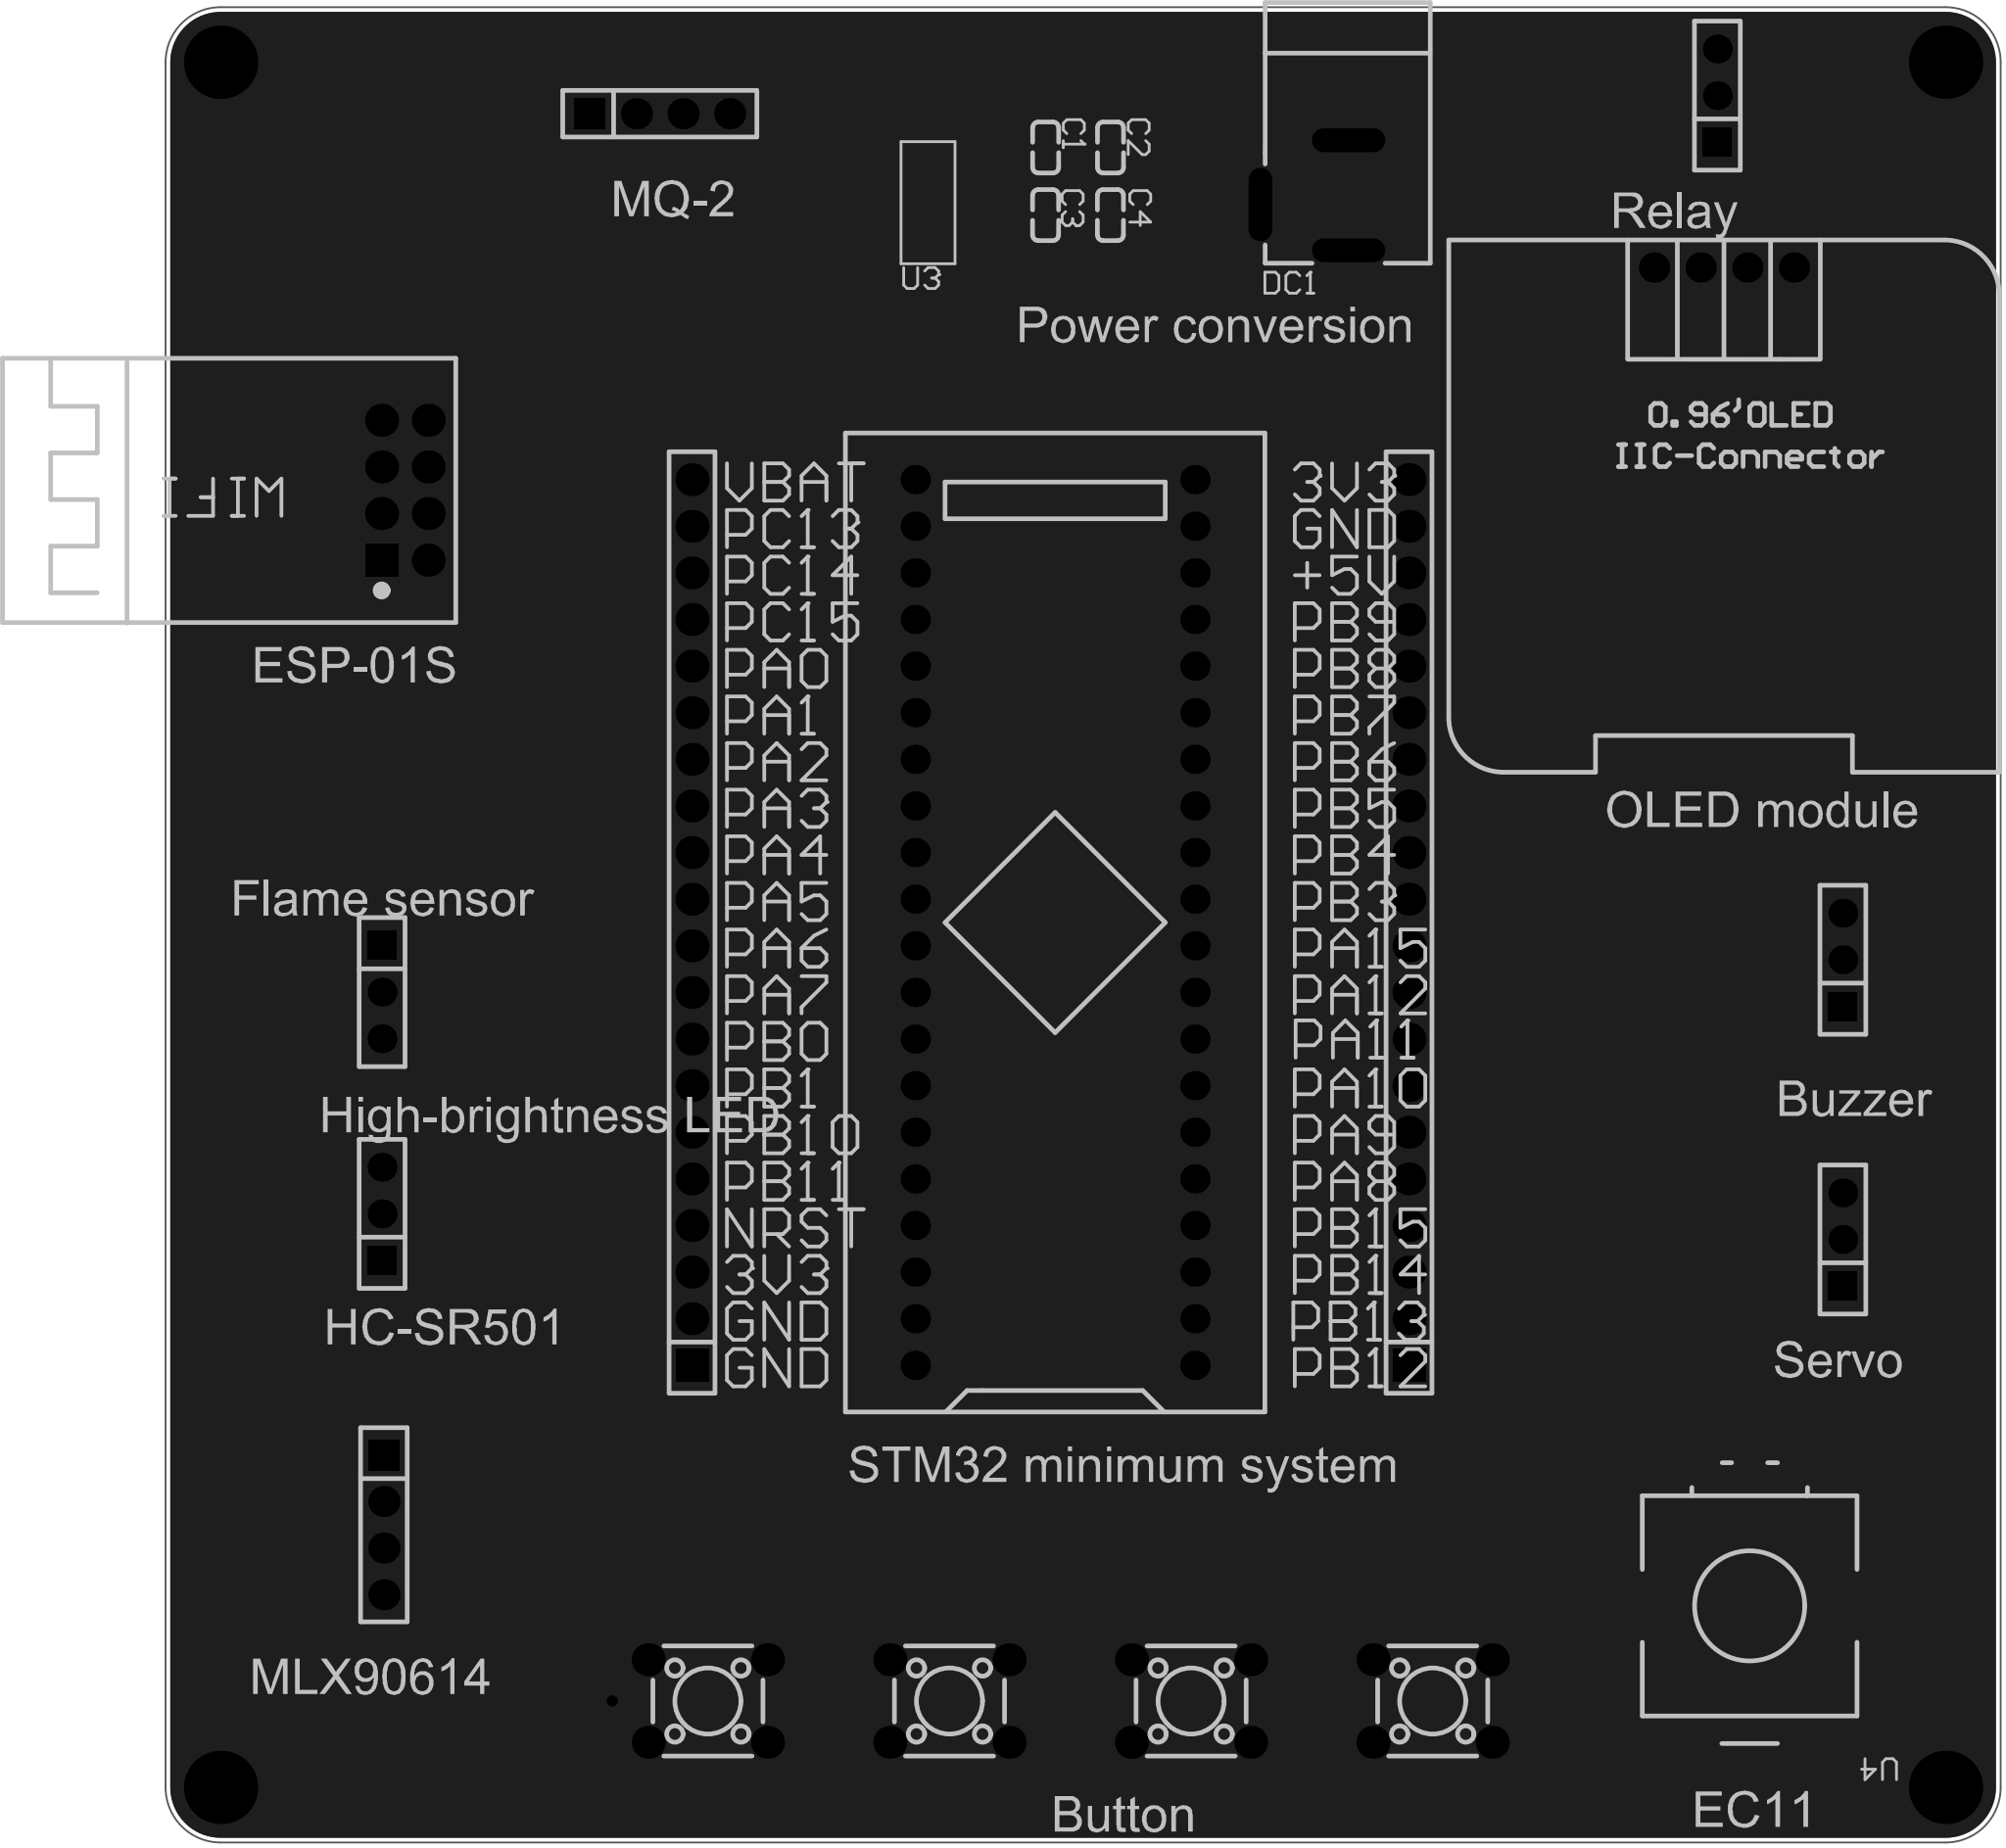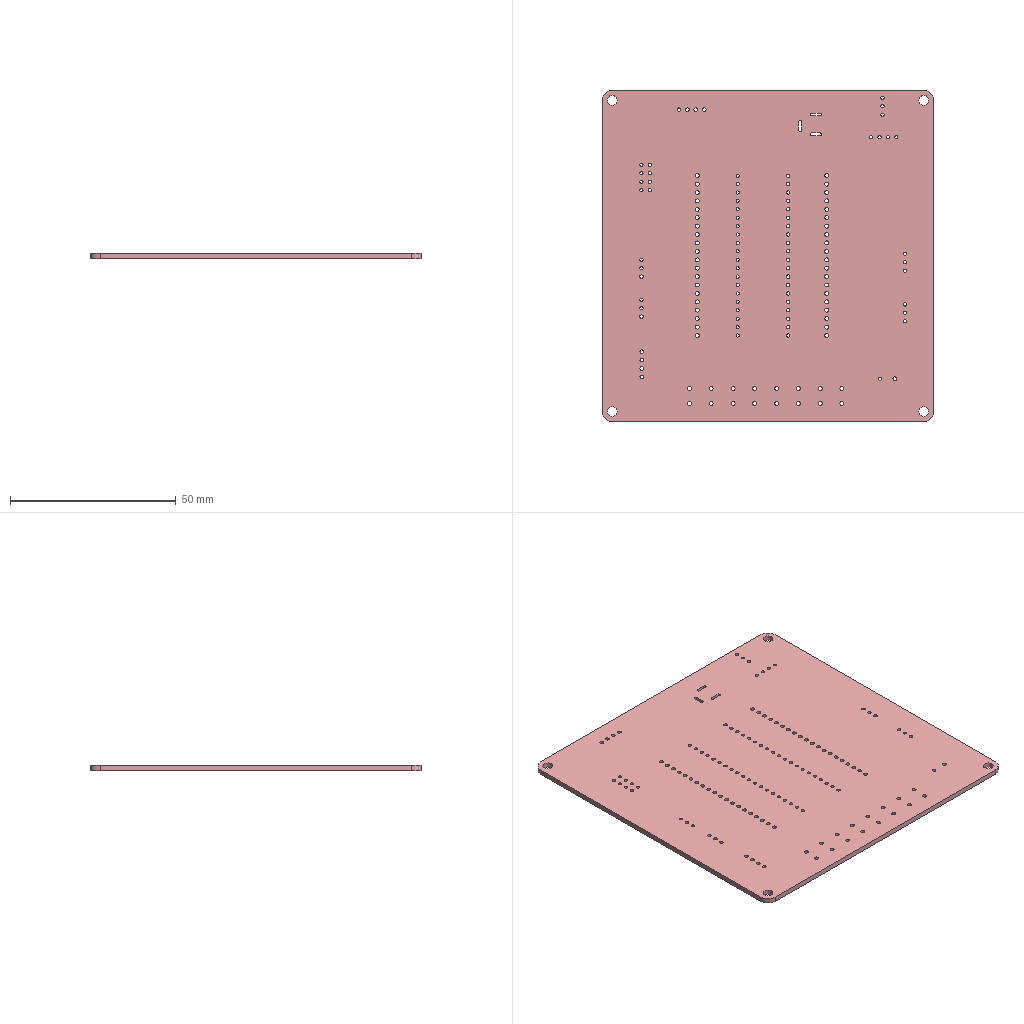Circuit board layout | Altium Designer | box 100 x 100 x 1.6 mm
Layer stack:
# Altium Designer layer stack of  (unit mm; dielectric type: 0 none, 1 core, 2 prepreg, 3 surface material)
index,name,kind,layer,copper_thickness_mm,dielectric_type,dielectric_thickness_mm,dielectric_material,dielectric_constant
0,Top Paste Mask Layer,other,,,,,,
1,Top Silkscreen Layer,other,,,,,,
2,Top Solder Mask Layer,dielectric,,,3,0.01,,3.3
3,Top Layer,copper,Top Layer,0.035,,,,
4,Dielectric1,dielectric,,,3,1.51,FR4,4.5
5,Bottom Layer,copper,Bottom Layer,0.035,,,,
6,Bottom Solder Mask Layer,dielectric,,,3,0.01,,3.3
7,Bottom Silkscreen Layer,other,,,,,,
8,Bottom Paste Mask Layer,other,,,,,,
# drill layer pairs: low layer,high layer
drill_pair,Top Layer,Bottom Layer
Part placement:
Designator,Comment,Layer,Footprint,Center-X(mm),Center-Y(mm),Rotation
U1,STM32F103C8T6-Card,TopLayer,CONN-TH_L53.3-W22.9_STM32F103C8T6-CARD,133.623,129.032,90
H1,,TopLayer,HDR-TH_20P-P2.54-V-F,152.906,129.032,90
H2,,TopLayer,HDR-TH_20P-P2.54-V-F,113.835,129.032,90
OLED1,,TopLayer,0.96OLED_4P,170.072,164.719,0
SW5,,TopLayer,SW-TH_4P-L6.0-W6.0-P4.50-LS6.5,154.197,86.614,0
SW6,,TopLayer,SW-TH_4P-L6.0-W6.0-P4.50-LS6.5,127.866,86.614,0
SW7,,TopLayer,SW-TH_4P-L6.0-W6.0-P4.50-LS6.5,114.7,86.614,0
U2,Ai-Thinker ESP-01S ESP8266,TopLayer,WIFIM-TH_8P-L24.7-W14.4-P2.54,98.19,152.585,180
H10,,TopLayer,HDR-TH_3P-P2.54-V-F,96.945,125.24,270
H11,,TopLayer,HDR-TH_3P-P2.54-V-F,96.945,113.157,90
H12,,TopLayer,HDR-TH_3P-P2.54-V-F,169.71,174.088,90
H13,,TopLayer,HDR-TH_3P-P2.54-V-F,176.549,111.76,90
H6,,TopLayer,HDR-TH_4P-P2.54-V-F,112.078,173.101,0
SW1,,TopLayer,SW-TH_4P-L6.0-W6.0-P4.50-LS6.5,141.031,86.614,0
C1,100nF,TopLayer,C0603,133.105,171.26,270
C2,100nF,TopLayer,C0603,136.639,171.26,270
C3,100nF,TopLayer,C0603,133.101,167.577,90
C4,100nF,TopLayer,C0603,136.635,167.577,90
U3,AMS1117-3.3,TopLayer,SOT-223-3_L6.5-W3.4-P2.30-LS7.0-BR,126.794,168.252,0
DC1,,TopLayer,DC-2.0,147.212,168.656,90
H4,,TopLayer,HDR-TH_3P-P2.54-V-F,176.549,127,90
H5,,TopLayer,HDR-TH_4P-P2.54-V-F,97.044,96.216,270
U4,EC1106S,TopLayer,SW-SMD_EC1106S,171.469,91.948,180
Pad and via stacks:
# Altium Designer via and pad stacks of  (unit mm). Each distinct definition once, with the count of objects using it.
# via: kind,start_layer,end_layer,hole_mm,diameter_mm,mode(0 simple;1 top-mid-bottom;2 full stack),diameter_per_layer,count,example_net
# pad: kind,layer,hole_mm,hole_type(0 round;1 square;2 slot),plating,top_size,top_shape(1 round;2 rect;3 octagon;9 rounded rect),mid_size,bottom_size,mode,footprint,size_per_layer,count,example
pad,Multi-Layer,3,0,plated,4x4,1,4x4,4x4,0,,,4,1
pad,Multi-Layer,1,0,plated,1.6x1.6,1,1.6x1.6,1.6x1.6,0,CONN-TH_L53.3-W22.9_STM32F103C8T6-CARD,,40,U1.1
pad,Multi-Layer,1.2,0,plated,1.8x1.8,2,1.8x1.8,1.8x1.8,0,HDR-TH_20P-P2.54-V-F,,2,H1.1
pad,Multi-Layer,1.2,0,plated,1.8x1.8,1,1.8x1.8,1.8x1.8,0,HDR-TH_20P-P2.54-V-F,,38,H1.2
pad,Multi-Layer,1,0,plated,1.65x1.65,1,1.65x1.65,1.65x1.65,0,0.96OLED_4P,,4,OLED1.4
pad,Multi-Layer,1.2,0,plated,1.8x1.8,1,1.8x1.8,1.8x1.8,0,SW-TH_4P-L6.0-W6.0-P4.50-LS6.5,,16,SW5.1
pad,Multi-Layer,1,0,plated,1.8x1.8,1,1.8x1.8,1.8x1.8,0,WIFIM-TH_8P-L24.7-W14.4-P2.54,,7,U2.8
pad,Multi-Layer,1,0,plated,1.8x1.8,2,1.8x1.8,1.8x1.8,0,WIFIM-TH_8P-L24.7-W14.4-P2.54,,1,U2.1
pad,Multi-Layer,1.02,0,plated,1.575x1.575,1,1.575x1.575,1.575x1.575,0,HDR-TH_3P-P2.54-V-F,,10,H10.3
pad,Multi-Layer,1.02,0,plated,1.575x1.575,2,1.575x1.575,1.575x1.575,0,HDR-TH_3P-P2.54-V-F,,5,H10.1
pad,Multi-Layer,1.1,0,plated,1.7x1.7,2,1.7x1.7,1.7x1.7,0,HDR-TH_4P-P2.54-V-F,,2,H6.1
pad,Multi-Layer,1.1,0,plated,1.7x1.7,1,1.7x1.7,1.7x1.7,0,HDR-TH_4P-P2.54-V-F,,6,H6.2
pad,Multi-Layer,0.8001,2,plated,4x1.3,1,4x1.3,4x1.3,0,DC-2.0,,3,DC1.2
pad,Top Layer,0,0,plated,0.8x0.9,2,0.8x0.9,0.8x0.9,0,C0603,,8,C1.2
pad,Top Layer,0,0,plated,2.5x1.1,2,2.5x1.1,2.5x1.1,0,SOT-223-3_L6.5-W3.4-P2.30-LS7.0-BR,,3,U3.1
pad,Top Layer,0,0,plated,2.34x3.6,2,2.34x3.6,2.34x3.6,0,SOT-223-3_L6.5-W3.4-P2.30-LS7.0-BR,,1,U3.4
pad,Top Layer,0,0,plated,1.5x1.8,2,1.5x1.8,1.5x1.8,0,SW-SMD_EC1106S,,5,U4.1
pad,Top Layer,0,0,plated,2.5x3.5,2,2.5x3.5,2.5x3.5,0,SW-SMD_EC1106S,,2,U4.6
via,Top Layer,Bottom Layer,0.3048,0.61,0,,1,GND
Copper pours:
name,layer,net,type(0 solid;1 hatched;2 none)
Bottom Layer-GND,Bottom Layer,GND,0
Top Layer-GND,Top Layer,GND,0